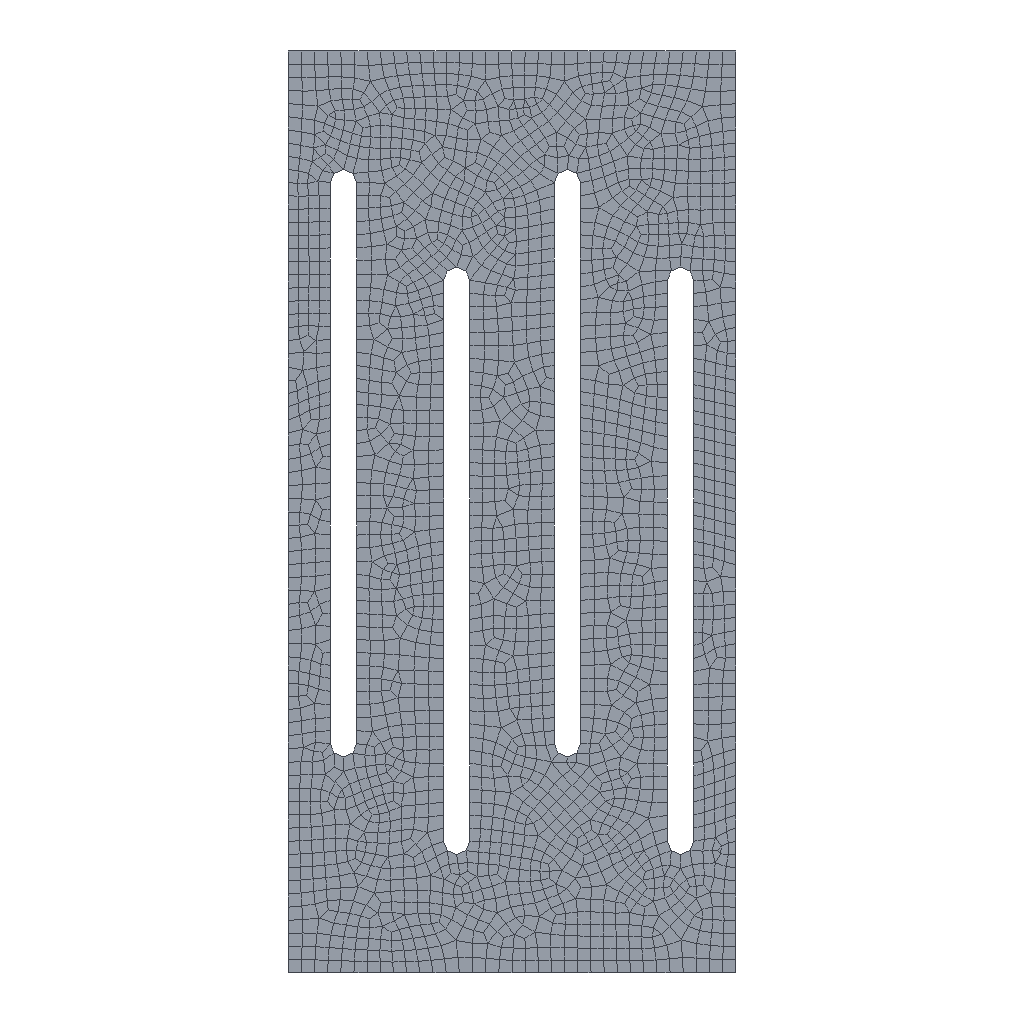Simulation study | abaqus
Set-up summary:
category,name,step,type,value,unit,region
solver,abaqus,,Abaqus/CAE 2024
units,unstated,,unstated,E=3.433 density= (no match)
analysis,Step-1,,static,time_period=1
mesh,nodes,,,2723
mesh,elements,,,2472
element_type,CPS4R,,,2394
element_type,CPS3,,,78
material,Material-1,,E,3.433
material,Material-1,,nu,0.13
material,Material-1,,yield,0.3282
material,Material-1,,behaviors,plastic
section,Material-1,,solid section,,,Set-1
bc,BC-3,initial,fixed,"[dofs=rz,x,y n=3]",,_PickedSet20
bc,BC-2,Step-1,fixed,"[dofs=rz,x n=2]",,Set-6
bc,BC-2,Step-1,displacement,35 [dofs=y],,Set-6
contact,Int-1,initial,contact pair surface to surface,interaction=IntProp-1; friction=0.1; behavior=hard,,_PickedSurf16 /
constraint,coupling,,,1
Abaqus input file, long lists of numbers shortened:
*Heading
** Job name: deck Model name: Model-1-Copy
** Generated by: Abaqus/CAE 2024
*Preprint, echo=NO, model=NO, history=NO, contact=NO
**
** PARTS
**
*Part, name=P2
*End Part
**
**
** ASSEMBLY
**
*Assembly, name=Assembly
**
*Instance, name=P2-1, part=P2
*Node
      1,   -8.954,   1.654
      2,  -8.6,   1.8
** (2720 more lines like these left out)
*Element, type=CPS3
 1, 2140, 1930, 1985
 2, 2326, 2648, 1791
** (76 more lines like these left out)
*Element, type=CPS4R
  79,  981, 1348,    1,    2
  80,    1, 1348, 1001,    4
** (2392 more lines like these left out)
*Nset, nset=Set-1, generate
    1,  2722,     1
*Elset, elset=Set-1, generate
    1,  2472,     1
** Section: Section-1
*Solid Section, elset=Set-1, material=Material-1
,
*End Instance
**
*Node
      1,         -6.5,          10.,           0.
*Nset, nset=Set-3, instance=P2-1
 227, 228, 229, 230, 231, 232, 233, 234, 235, 236, 237, 238, 239, 240, 241, 242
 243, 905, 906, 907, 908, 909, 910, 911, 912, 913, 914, 915, 916, 917, 918, 919
** (1 more lines like these left out)
*Elset, elset=Set-3, instance=P2-1
  150,  151,  152,  153,  222,  223,  237,  255,  257,  413,  414,  684,  692,  693,  699,  700
  704,  705,  709,  714,  717,  720, 1194, 1195, 1199, 1322, 1326, 1327, 1365, 1366, 1370, 1372
** (1 more lines like these left out)
*Nset, nset=Set-4, instance=P2-1
 226, 277, 278, 279, 280, 281, 282, 283, 284, 285, 286, 287, 288, 289, 290, 291
 292, 959, 960, 961, 962, 963, 964, 965, 966, 967, 968, 969, 970, 971, 972, 973
** (1 more lines like these left out)
*Elset, elset=Set-4, instance=P2-1
   98,  100,  185,  186,  187,  371,  372,  373,  374,  386,  387,  447,  448,  449,  450,  637
  721,  730,  738,  739,  745,  754,  760, 1233, 1237, 1240, 1319, 1377, 1378, 1379, 1381, 1383
** (1 more lines like these left out)
*Nset, nset=Set-6
 1,
*Nset, nset=m_Set-5
 1,
*Nset, nset=_PickedSet19, internal, instance=P2-1
 226, 227
*Nset, nset=_PickedSet20, internal, instance=P2-1
 227, 228, 229, 230, 231, 232, 233, 234, 235, 236, 237, 238, 239, 240, 241, 242
 243, 905, 906, 907, 908, 909, 910, 911, 912, 913, 914, 915, 916, 917, 918, 919
** (1 more lines like these left out)
*Elset, elset=_PickedSet20, internal, instance=P2-1
  150,  151,  152,  153,  222,  223,  237,  255,  257,  413,  414,  684,  692,  693,  699,  700
  704,  705,  709,  714,  717,  720, 1194, 1195, 1199, 1322, 1326, 1327, 1365, 1366, 1370, 1372
** (1 more lines like these left out)
*Nset, nset=_PickedSet21, internal, instance=P2-1
 226, 277, 278, 279, 280, 281, 282, 283, 284, 285, 286, 287, 288, 289, 290, 291
 292, 959, 960, 961, 962, 963, 964, 965, 966, 967, 968, 969, 970, 971, 972, 973
** (1 more lines like these left out)
*Nset, nset=_PickedSet21, internal
 1,
*Elset, elset=_PickedSet21, internal, instance=P2-1
   98,  100,  185,  186,  187,  371,  372,  373,  374,  386,  387,  447,  448,  449,  450,  637
  721,  730,  738,  739,  745,  754,  760, 1233, 1237, 1240, 1319, 1377, 1378, 1379, 1381, 1383
** (1 more lines like these left out)
*Elset, elset=_s_Surf-1_S1, internal, instance=P2-1
   98,  100,  185,  187,  386,  447,  448,  449,  450,  721,  730,  738,  745,  754,  760, 1319
 1377, 1378, 1381, 1383
*Elset, elset=_s_Surf-1_S4, internal, instance=P2-1
  186,  387,  637, 1237, 1240
*Elset, elset=_s_Surf-1_S2, internal, instance=P2-1, generate
 371,  374,    1
*Elset, elset=_s_Surf-1_S3, internal, instance=P2-1
  739, 1233, 1379, 1385, 1465
*Surface, type=ELEMENT, name=s_Surf-1
_s_Surf-1_S1, S1
_s_Surf-1_S4, S4
_s_Surf-1_S2, S2
_s_Surf-1_S3, S3
*Elset, elset=__PickedSurf16_S3, internal, instance=P2-1
   79,   89,  208,  304,  310,  315,  316,  321,  322,  327,  328,  332,  345,  351,  357,  364
  369,  436,  442,  444,  534,  572,  573,  574,  575,  595,  596,  641,  657,  664,  792, 1076
** (1 more lines like these left out)
*Elset, elset=__PickedSurf16_S4, internal, instance=P2-1
   80,  128,  129,  130,  131,  139,  194,  198,  200,  231,  238,  240,  274,  283,  288,  292
  295,  301,  303,  325,  326,  416,  417,  418,  419,  443,  465,  466,  470,  473,  479,  485
** (3 more lines like these left out)
*Elset, elset=__PickedSurf16_S2, internal, instance=P2-1
   83,   84,   86,  132,  133,  134,  135,  136,  137,  138,  141,  142,  143,  144,  201,  202
  203,  204,  205,  206,  207,  210,  211,  213,  215,  224,  232,  239,  244,  247,  275,  307
** (8 more lines like these left out)
*Elset, elset=__PickedSurf16_S1, internal, instance=P2-1
   85,  111,  112,  113,  114,  115,  195,  199,  212,  241,  266,  267,  268,  269,  270,  280
  286,  290,  293,  298,  314,  320,  350,  353,  363,  366,  378,  394,  400,  401,  415,  421
** (5 more lines like these left out)
*Surface, type=ELEMENT, name=_PickedSurf16, internal
__PickedSurf16_S3, S3
__PickedSurf16_S4, S4
__PickedSurf16_S2, S2
__PickedSurf16_S1, S1
*Surface, type=NODE, name=_PickedSet21_CNS_, internal
_PickedSet21, 1.
** Constraint: Constraint-1
*Coupling, constraint name=Constraint-1, ref node=m_Set-5, surface=_PickedSet21_CNS_
*Kinematic
*End Assembly
**
** MATERIALS
**
*Material, name=Material-1
*Elastic
 3.433, 0.13
*Plastic
 0.3282,         0.
 0.3322,  0.005767
 0.3376, 0.005993
 0.3423, 0.006387
  0.3465, 0.006957
 0.3514, 0.007303
 0.3568, 0.007534
 0.3608, 0.008123
 0.3655,  0.008548
 0.3704, 0.008898
 0.3756, 0.009164
 0.3794, 0.009839
 0.3854,   0.009885
 0.3888,  0.01065
 0.3939,  0.01097
 0.398,  0.01156
 0.4034,   0.01174
 0.4078,  0.01224
 0.4116,  0.01294
 0.4165,  0.0133
 0.421,  0.01376
 0.4263,  0.01401
 0.4293,  0.0149
 0.435,   0.01503
 0.4394,  0.01554
 0.4429,  0.01628
 0.448,  0.01657
 0.4531,  0.01689
 0.4572,  0.01748
 0.4609,  0.01817
 0.4657,  0.01856
 0.4705,  0.01892
 0.4748,  0.01945
 0.4779,   0.02033
 0.4885,  0.02082
 0.4912,  0.02181
 0.4968,  0.02197
 0.5012,  0.02245
 0.5054,  0.02301
 0.5094,  0.02363
** (2281 more lines like these left out)
**
** INTERACTION PROPERTIES
**
*Surface Interaction, name=IntProp-1
1.,
*Friction, slip tolerance=0.005
 0.1,
*Surface Behavior, pressure-overclosure=HARD
**
** BOUNDARY CONDITIONS
**
** Name: BC-3 Type: Displacement/Rotation
*Boundary
_PickedSet20, 1, 1
_PickedSet20, 2, 2
_PickedSet20, 6, 6
**
** INTERACTIONS
**
** Interaction: Int-1
*Contact Pair, interaction=IntProp-1, type=SURFACE TO SURFACE
_PickedSurf16,
** ----------------------------------------------------------------
**
** STEP: Step-1
**
*Step, name=Step-1, nlgeom=NO, inc=10000
*Static
0.01, 1., 1e-05, 0.05
**
** BOUNDARY CONDITIONS
**
** Name: BC-2 Type: Displacement/Rotation
*Boundary
Set-6, 1, 1
Set-6, 2, 2, 35.
Set-6, 6, 6
**
** OUTPUT REQUESTS
**
*Restart, write, frequency=0
**
** FIELD OUTPUT: F-Output-1
**
*Output, field, variable=PRESELECT
**
** HISTORY OUTPUT: H-Output-1
**
*Output, history, variable=PRESELECT
*End Step
Results summary:
result,odb.job_status,,,JOB_STATUS_COMPLETED_SUCCESSFULLY,"consistent, unstated (Abaqus has no unit system)"
result,steps[0].procedure,Step-1,,*STATIC,"consistent, unstated (Abaqus has no unit system)"
result,steps[0].time_period,Step-1,,1,"consistent, unstated (Abaqus has no unit system)"
result,steps[0].n_frames,Step-1,,108,"consistent, unstated (Abaqus has no unit system)"
result,steps[0].last_frame.id,Step-1,,107,"consistent, unstated (Abaqus has no unit system)"
result,steps[0].last_frame.value,Step-1,,1,"consistent, unstated (Abaqus has no unit system)"
result,steps[0].last_frame.description,Step-1,,Increment    107: Step Time =    1.000,"consistent, unstated (Abaqus has no unit system)"
result,steps[0].completed,Step-1,,True,"consistent, unstated (Abaqus has no unit system)"
result,steps[0].max_U_magnitude,Step-1,,35,"consistent, unstated (Abaqus has no unit system)"
result,steps[0].max_S_mises,Step-1,,2.567,"consistent, unstated (Abaqus has no unit system)"
result,steps[0].RF_sum[1],Step-1,,-4.47035e-08,"consistent, unstated (Abaqus has no unit system)"
result,steps[0].RF_sum[2],Step-1,,-2.74181e-06,"consistent, unstated (Abaqus has no unit system)"